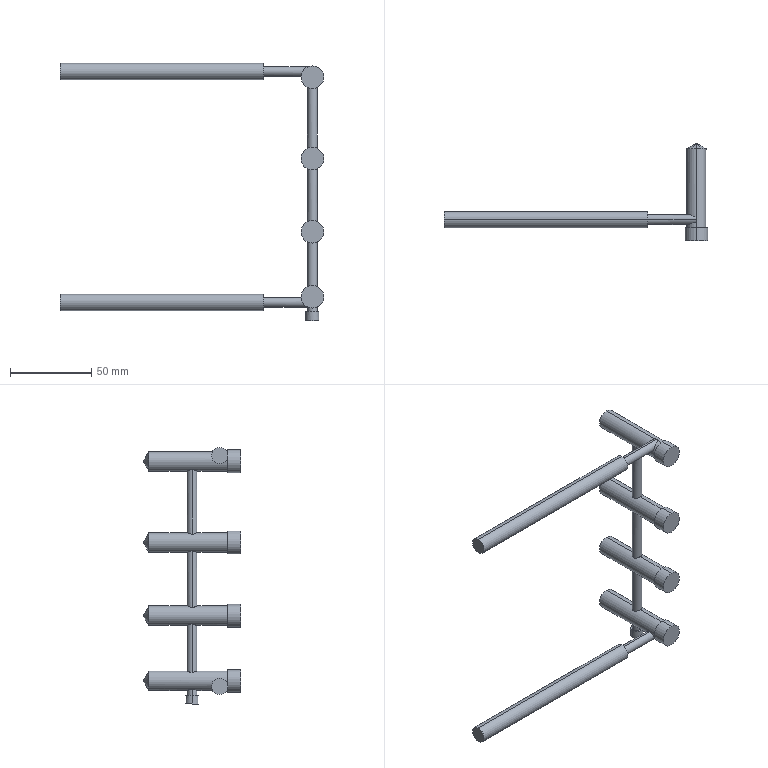Part | STEP file | 1 solid | 58 faces | box 162 x 60 x 158.144 mm | volume 51671 mm3 | cylinder 35 | plane 15 | cone 8 | commonest cylinder face diameters 6 x13 12 x8 14 x8 10 x4 8 x2